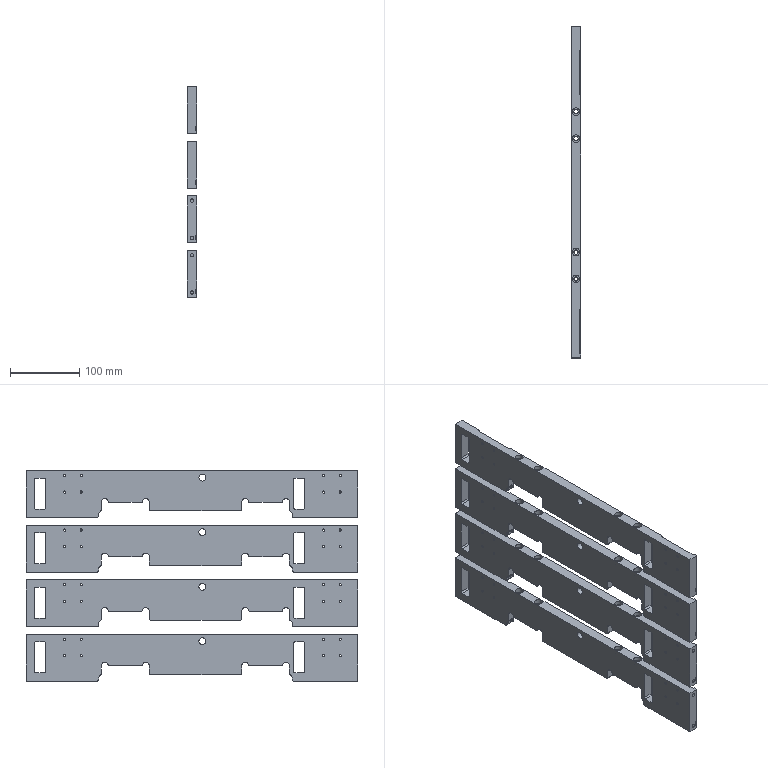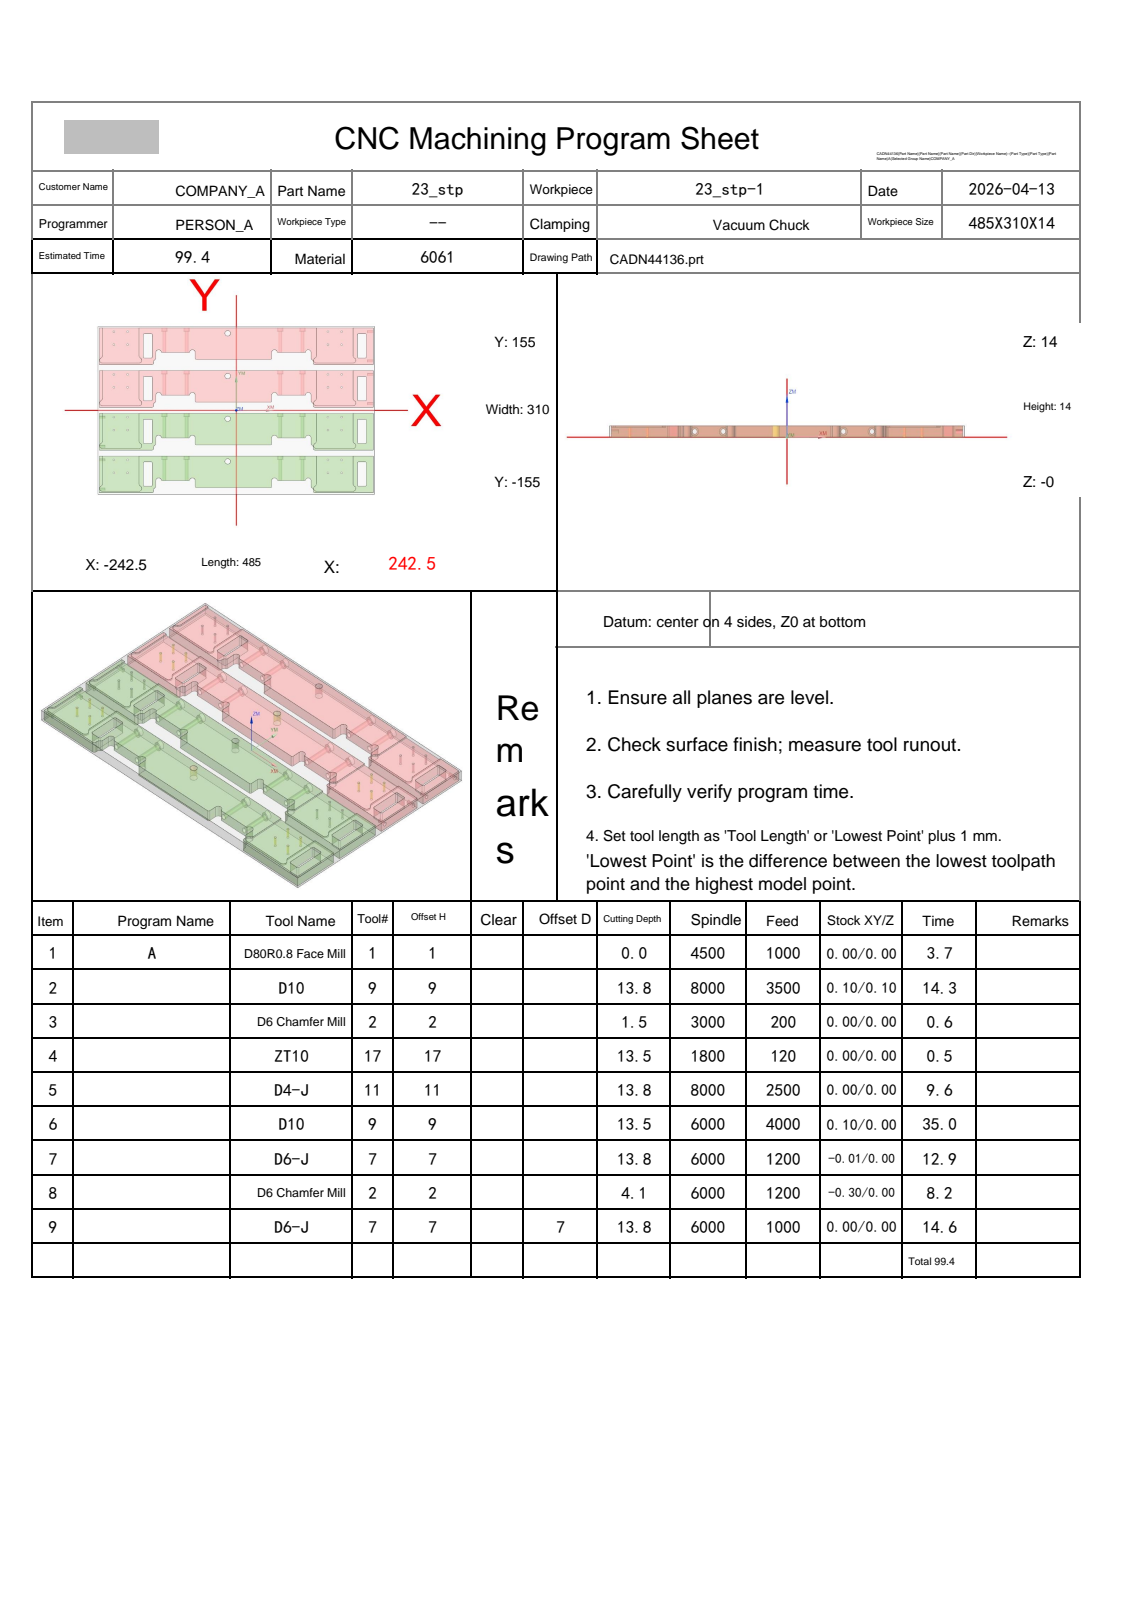NC program | NX | posted by the shop | part box 14 x 480 x 305 mm
Lines 1 to 2632 of 51894:
%
O0001
(Machine time: 100.72 MIN)
(===Total Tool:6===)
(T1=D80R0.8 Face Mill D=80.  R=0.8  D-  H01 Z=14.   )
(T9=D10     D=10.  R=0.   D-  H09 Z=0.2   )
(T2=D6 Chamfer Mill   D=6.   R=0.   D-  H02 Z=9.85  )
(T17=ZT10   D=10.  DR_a=118 D-  H17 Z=0.5   )
(T11=D4-J   D=4.   R=0.   D11 H11 Z=0.2   )
(T7=D6-J    D=6.   R=0.   D7  H07 Z=0.2   )
G80 G90 G17 G49 G40
G91 G28 Z0
M01
N1 T01 M06
(D80R0.8 Face Mill  D=80. R=0.8 H=01 ce=0.00 di=0.00)
G00 G90 G54 X-292. Y137.5 M03 S4500
G43 H01 Z34.
M08
Z16.
G01 Z14. F1000.
X-280.
X280.
Y82.5
X-280.
Y27.5
X280.
Y-27.5
X-280.
Y-82.5
X280.
Y-137.5
X-280.
X-292.
Z16.
G00 Z34.
G91 G28 Z0.0
M05
M09
G91 G28 Z0.0
M01
N2 T09 M06
(D10  D=10. R=0. H=09 ce=0.10 di=0.10)
G00 G90 G54 X-201.35 Y-115.71 M03 S8000
G43 H09 Z34.
M08
Z14.5
M03 S8000
G01 Y-110.28 Z14.31 F2800.
X-203.65 Z14.23
Y-118.65 Z13.938
X-201.35 Z13.857
Y-110.28 Z13.565
X-202.5 Z13.525
Y-109.98
M03 S8000
X-203.95 F3500.
Y-118.95
X-201.05
Y-109.98
X-202.5
Y-105.48
X-208.45
Y-123.45
X-196.55
Y-105.48
X-202.5
Y-98.48
X-215.45
Y-130.45
X-189.55
Y-98.48
X-202.5
Y-91.48
X-222.45
Y-135.84
G02 X-222.526 Y-137.45 I-17.05 J0.0
G01 X-182.474
G02 X-182.55 Y-135.84 I16.974 J1.61
G01 Y-91.48
X-202.5
Y-84.48
X-229.45
Y-135.84
G02 X-234.317 Y-144.45 I-10.05 J0.0
G01 X-170.701
X-171.032 Y-144.23
X-171.094 Y-144.189
G02 X-175.55 Y-135.84 I5.594 J8.349
G01 Y-84.48
X-202.5
Z14.525
G00 Z15.
X-201.35 Y-115.71
Z14.025
M03 S8000
G01 Y-110.28 Z13.835 F2800.
X-203.65 Z13.755
Y-118.65 Z13.463
X-201.35 Z13.382
Y-110.28 Z13.09
X-202.5 Z13.05
Y-109.98
M03 S8000
X-203.95 F3500.
Y-118.95
X-201.05
Y-109.98
X-202.5
Y-105.48
X-208.45
Y-123.45
X-196.55
Y-105.48
X-202.5
Y-98.48
X-215.45
Y-130.45
X-189.55
Y-98.48
X-202.5
Y-91.48
X-222.45
Y-135.84
G02 X-222.526 Y-137.45 I-17.05 J0.0
G01 X-182.474
G02 X-182.55 Y-135.84 I16.974 J1.61
G01 Y-91.48
X-202.5
Y-84.48
X-229.45
Y-135.84
G02 X-234.317 Y-144.45 I-10.05 J0.0
G01 X-170.701
X-171.032 Y-144.23
G02 X-175.55 Y-135.84 I5.532 J8.39
G01 Y-84.48
X-202.5
Z14.05
G00 Z14.525
X-201.35 Y-115.71
Z13.55
M03 S8000
G01 Y-110.28 Z13.36 F2800.
X-203.65 Z13.28
Y-118.65 Z12.988
X-201.35 Z12.907
Y-110.28 Z12.615
X-202.5 Z12.575
Y-109.98
M03 S8000
X-203.95 F3500.
Y-118.95
X-201.05
Y-109.98
X-202.5
Y-105.48
X-208.45
Y-123.45
X-196.55
Y-105.48
X-202.5
Y-98.48
X-215.45
Y-130.45
X-189.55
Y-98.48
X-202.5
Y-91.48
X-222.45
Y-135.84
G02 X-222.526 Y-137.45 I-17.05 J0.0
G01 X-182.474
G02 X-182.55 Y-135.84 I16.974 J1.61
G01 Y-91.48
X-202.5
Y-84.48
X-229.45
Y-135.84
G02 X-234.317 Y-144.45 I-10.05 J0.0
G01 X-170.701
X-171.032 Y-144.23
G02 X-175.55 Y-135.84 I5.532 J8.39
G01 Y-84.48
X-202.5
Z13.575
G00 Z14.05
X-201.35 Y-115.71
Z13.075
M03 S8000
G01 Y-110.28 Z12.885 F2800.
X-203.65 Z12.805
Y-118.65 Z12.513
X-201.35 Z12.432
Y-110.28 Z12.14
X-202.5 Z12.1
Y-109.98
M03 S8000
X-203.95 F3500.
Y-118.95
X-201.05
Y-109.98
X-202.5
Y-105.48
X-208.45
Y-123.45
X-196.55
Y-105.48
X-202.5
Y-98.48
X-215.45
Y-130.45
X-189.55
Y-98.48
X-202.5
Y-91.48
X-222.45
Y-135.84
G02 X-222.526 Y-137.45 I-17.05 J0.0
G01 X-182.474
G02 X-182.55 Y-135.84 I16.974 J1.61
G01 Y-91.48
X-202.5
Y-84.48
X-229.45
Y-135.84
G02 X-234.317 Y-144.45 I-10.05 J0.0
G01 X-170.701
X-171.032 Y-144.23
G02 X-175.55 Y-135.84 I5.532 J8.39
G01 Y-84.48
X-202.5
Z13.1
G00 Z34.
X-201.35 Y-36.71
Z14.5
M03 S8000
G01 Y-31.28 Z14.31 F2800.
X-203.65 Z14.23
Y-39.65 Z13.938
X-201.35 Z13.857
Y-31.28 Z13.565
X-202.5 Z13.525
Y-30.98
M03 S8000
X-203.95 F3500.
Y-39.95
X-201.05
Y-30.98
X-202.5
Y-26.48
X-208.45
Y-44.45
X-196.55
Y-26.48
X-202.5
Y-19.48
X-215.45
Y-51.45
X-189.55
Y-19.48
X-202.5
Y-12.48
X-222.45
Y-56.84
G02 X-222.526 Y-58.45 I-17.05 J0.0
G01 X-182.474
G02 X-182.55 Y-56.84 I16.974 J1.61
G01 Y-12.48
X-202.5
Y-5.48
X-229.45
Y-56.84
G02 X-234.317 Y-65.45 I-10.05 J0.0
G01 X-170.691
X-170.888 Y-65.323
G02 X-175.55 Y-56.84 I5.388 J8.483
G01 Y-5.48
X-202.5
Z14.525
G00 Z15.
X-201.35 Y-36.71
Z14.025
M03 S8000
G01 Y-31.28 Z13.835 F2800.
X-203.65 Z13.755
Y-39.65 Z13.463
X-201.35 Z13.382
Y-31.28 Z13.09
X-202.5 Z13.05
Y-30.98
M03 S8000
X-203.95 F3500.
Y-39.95
X-201.05
Y-30.98
X-202.5
Y-26.48
X-208.45
Y-44.45
X-196.55
Y-26.48
X-202.5
Y-19.48
X-215.45
Y-51.45
X-189.55
Y-19.48
X-202.5
Y-12.48
X-222.45
Y-56.84
G02 X-222.526 Y-58.45 I-17.05 J0.0
G01 X-182.474
G02 X-182.55 Y-56.84 I16.974 J1.61
G01 Y-12.48
X-202.5
Y-5.48
X-229.45
Y-56.84
G02 X-234.317 Y-65.45 I-10.05 J0.0
G01 X-170.691
X-170.888 Y-65.323
G02 X-175.55 Y-56.84 I5.388 J8.483
G01 Y-5.48
X-202.5
Z14.05
G00 Z14.525
X-201.35 Y-36.71
Z13.55
M03 S8000
G01 Y-31.28 Z13.36 F2800.
X-203.65 Z13.28
Y-39.65 Z12.988
X-201.35 Z12.907
Y-31.28 Z12.615
X-202.5 Z12.575
Y-30.98
M03 S8000
X-203.95 F3500.
Y-39.95
X-201.05
Y-30.98
X-202.5
Y-26.48
X-208.45
Y-44.45
X-196.55
Y-26.48
X-202.5
Y-19.48
X-215.45
Y-51.45
X-189.55
Y-19.48
X-202.5
Y-12.48
X-222.45
Y-56.84
G02 X-222.526 Y-58.45 I-17.05 J0.0
G01 X-182.474
G02 X-182.55 Y-56.84 I16.974 J1.61
G01 Y-12.48
X-202.5
Y-5.48
X-229.45
Y-56.84
G02 X-234.317 Y-65.45 I-10.05 J0.0
G01 X-170.691
X-170.888 Y-65.323
G02 X-175.55 Y-56.84 I5.388 J8.483
G01 Y-5.48
X-202.5
Z13.575
G00 Z14.05
X-201.35 Y-36.71
Z13.075
M03 S8000
G01 Y-31.28 Z12.885 F2800.
X-203.65 Z12.805
Y-39.65 Z12.513
X-201.35 Z12.432
Y-31.28 Z12.14
X-202.5 Z12.1
Y-30.98
M03 S8000
X-203.95 F3500.
Y-39.95
X-201.05
Y-30.98
X-202.5
Y-26.48
X-208.45
Y-44.45
X-196.55
Y-26.48
X-202.5
Y-19.48
X-215.45
Y-51.45
X-189.55
Y-19.48
X-202.5
Y-12.48
X-222.45
Y-56.84
G02 X-222.526 Y-58.45 I-17.05 J0.0
G01 X-182.474
G02 X-182.55 Y-56.84 I16.974 J1.61
G01 Y-12.48
X-202.5
Y-5.48
X-229.45
Y-56.84
G02 X-234.317 Y-65.45 I-10.05 J0.0
G01 X-170.691
X-170.888 Y-65.323
G02 X-175.55 Y-56.84 I5.388 J8.483
G01 Y-5.48
X-202.5
Z13.1
G00 Z34.
X-201.35 Y42.29
Z14.5
M03 S8000
G01 Y47.72 Z14.31 F2800.
X-203.65 Z14.23
Y39.35 Z13.938
X-201.35 Z13.857
Y47.72 Z13.565
X-202.5 Z13.525
Y48.02
M03 S8000
X-203.95 F3500.
Y39.05
X-201.05
Y48.02
X-202.5
Y52.52
X-208.45
Y34.55
X-196.55
Y52.52
X-202.5
Y59.52
X-215.45
Y27.55
X-189.55
Y59.52
X-202.5
Y66.52
X-222.45
Y22.16
G02 X-222.526 Y20.55 I-17.05 J0.0
G01 X-182.474
G02 X-182.55 Y22.16 I16.974 J1.61
G01 Y66.52
X-202.5
Y73.52
X-229.45
Y22.16
G02 X-234.317 Y13.55 I-10.05 J0.0
G01 X-170.692
X-170.818 Y13.633
X-170.856 Y13.656
G02 X-175.55 Y22.16 I5.356 J8.504
G01 Y73.52
X-202.5
Z14.525
G00 Z15.
X-201.35 Y42.29
Z14.025
M03 S8000
G01 Y47.72 Z13.835 F2800.
X-203.65 Z13.755
Y39.35 Z13.463
X-201.35 Z13.382
Y47.72 Z13.09
X-202.5 Z13.05
Y48.02
M03 S8000
X-203.95 F3500.
Y39.05
X-201.05
Y48.02
X-202.5
Y52.52
X-208.45
Y34.55
X-196.55
Y52.52
X-202.5
Y59.52
X-215.45
Y27.55
X-189.55
Y59.52
X-202.5
Y66.52
X-222.45
Y22.16
G02 X-222.526 Y20.55 I-17.05 J0.0
G01 X-182.474
G02 X-182.55 Y22.16 I16.974 J1.61
G01 Y66.52
X-202.5
Y73.52
X-229.45
Y22.16
G02 X-234.317 Y13.55 I-10.05 J0.0
G01 X-170.692
X-170.818 Y13.633
G02 X-175.55 Y22.16 I5.318 J8.528
G01 Y73.52
X-202.5
Z14.05
G00 Z14.525
X-201.35 Y42.29
Z13.55
M03 S8000
G01 Y47.72 Z13.36 F2800.
X-203.65 Z13.28
Y39.35 Z12.988
X-201.35 Z12.907
Y47.72 Z12.615
X-202.5 Z12.575
Y48.02
M03 S8000
X-203.95 F3500.
Y39.05
X-201.05
Y48.02
X-202.5
Y52.52
X-208.45
Y34.55
X-196.55
Y52.52
X-202.5
Y59.52
X-215.45
Y27.55
X-189.55
Y59.52
X-202.5
Y66.52
X-222.45
Y22.16
G02 X-222.526 Y20.55 I-17.05 J0.0
G01 X-182.474
G02 X-182.55 Y22.16 I16.974 J1.61
G01 Y66.52
X-202.5
Y73.52
X-229.45
Y22.16
G02 X-234.317 Y13.55 I-10.05 J0.0
G01 X-170.692
X-170.818 Y13.633
G02 X-175.55 Y22.16 I5.318 J8.528
G01 Y73.52
X-202.5
Z13.575
G00 Z14.05
X-201.35 Y42.29
Z13.075
M03 S8000
G01 Y47.72 Z12.885 F2800.
X-203.65 Z12.805
Y39.35 Z12.513
X-201.35 Z12.432
Y47.72 Z12.14
X-202.5 Z12.1
Y48.02
M03 S8000
X-203.95 F3500.
Y39.05
X-201.05
Y48.02
X-202.5
Y52.52
X-208.45
Y34.55
X-196.55
Y52.52
X-202.5
Y59.52
X-215.45
Y27.55
X-189.55
Y59.52
X-202.5
Y66.52
X-222.45
Y22.16
G02 X-222.526 Y20.55 I-17.05 J0.0
G01 X-182.474
G02 X-182.55 Y22.16 I16.974 J1.61
G01 Y66.52
X-202.5
Y73.52
X-229.45
Y22.16
G02 X-233.984 Y13.76 I-10.05 J0.0
X-234.317 Y13.55 I-5.516 J8.401
G01 X-170.692
X-170.818 Y13.633
G02 X-175.55 Y22.16 I5.318 J8.528
G01 Y73.52
X-202.5
Z13.1
G00 Z34.
X-201.35 Y121.29
Z14.5
M03 S8000
G01 Y126.72 Z14.31 F2800.
X-203.65 Z14.23
Y118.35 Z13.938
X-201.35 Z13.857
Y126.72 Z13.565
X-202.5 Z13.525
Y127.02
M03 S8000
X-203.95 F3500.
Y118.05
X-201.05
Y127.02
X-202.5
Y131.52
X-208.45
Y113.55
X-196.55
Y131.52
X-202.5
Y138.52
X-215.45
Y106.55
X-189.55
Y138.52
X-202.5
Y145.52
X-222.45
Y101.16
G02 X-222.526 Y99.55 I-17.05 J0.0
G01 X-182.474
G02 X-182.55 Y101.16 I16.974 J1.61
G01 Y145.52
X-202.5
Y152.52
X-229.055
X-229.45
Y101.16
G02 X-234.317 Y92.55 I-10.05 J0.0
G01 X-170.701
X-171.061 Y92.789
G02 X-175.55 Y101.16 I5.561 J8.371
G01 Y152.52
X-202.5
Z14.525
G00 Z15.
X-201.35 Y121.29
Z14.025
M03 S8000
G01 Y126.72 Z13.835 F2800.
X-203.65 Z13.755
Y118.35 Z13.463
X-201.35 Z13.382
Y126.72 Z13.09
X-202.5 Z13.05
Y127.02
M03 S8000
X-203.95 F3500.
Y118.05
X-201.05
Y127.02
X-202.5
Y131.52
X-208.45
Y113.55
X-196.55
Y131.52
X-202.5
Y138.52
X-215.45
Y106.55
X-189.55
Y138.52
X-202.5
Y145.52
X-222.45
Y101.16
G02 X-222.526 Y99.55 I-17.05 J0.0
G01 X-182.474
G02 X-182.55 Y101.16 I16.974 J1.61
G01 Y145.52
X-202.5
Y152.52
X-229.055
X-229.45
Y101.16
G02 X-234.317 Y92.55 I-10.05 J0.0
G01 X-170.701
X-171.06 Y92.788
G02 X-175.55 Y101.16 I5.56 J8.372
G01 Y152.52
X-202.5
Z14.05
G00 Z14.525
X-201.35 Y121.29
Z13.55
M03 S8000
G01 Y126.72 Z13.36 F2800.
X-203.65 Z13.28
Y118.35 Z12.988
X-201.35 Z12.907
Y126.72 Z12.615
X-202.5 Z12.575
Y127.02
M03 S8000
X-203.95 F3500.
Y118.05
X-201.05
Y127.02
X-202.5
Y131.52
X-208.45
Y113.55
X-196.55
Y131.52
X-202.5
Y138.52
X-215.45
Y106.55
X-189.55
Y138.52
X-202.5
Y145.52
X-222.45
Y101.16
G02 X-222.526 Y99.55 I-17.05 J0.0
G01 X-182.474
G02 X-182.55 Y101.16 I16.974 J1.61
G01 Y145.52
X-202.5
Y152.52
X-229.055
X-229.45
Y101.16
G02 X-234.317 Y92.55 I-10.05 J0.0
G01 X-170.701
X-171.06 Y92.788
G02 X-175.55 Y101.16 I5.56 J8.372
G01 Y152.52
X-202.5
Z13.575
G00 Z14.05
X-201.35 Y121.29
Z13.075
M03 S8000
G01 Y126.72 Z12.885 F2800.
X-203.65 Z12.805
Y118.35 Z12.513
X-201.35 Z12.432
Y126.72 Z12.14
X-202.5 Z12.1
Y127.02
M03 S8000
X-203.95 F3500.
Y118.05
X-201.05
Y127.02
X-202.5
Y131.52
X-208.45
Y113.55
X-196.55
Y131.52
X-202.5
Y138.52
X-215.45
Y106.55
X-189.55
Y138.52
X-202.5
Y145.52
X-222.45
Y101.16
G02 X-222.526 Y99.55 I-17.05 J0.0
G01 X-182.474
G02 X-182.55 Y101.16 I16.974 J1.61
G01 Y145.52
X-202.5
Y152.52
X-229.055
X-229.45
Y101.16
G02 X-234.317 Y92.55 I-10.05 J0.0
G01 X-170.701
X-171.06 Y92.788
G02 X-175.55 Y101.16 I5.56 J8.372
G01 Y152.52
X-202.5
Z13.1
G00 Z34.
X173.65 Y121.29
Z14.5
M03 S8000
G01 Y126.72 Z14.31 F2800.
X171.35 Z14.23
Y118.35 Z13.938
X173.65 Z13.857
Y126.72 Z13.565
X172.5 Z13.525
Y127.02
M03 S8000
X171.05 F3500.
Y118.05
X173.95
Y127.02
X172.5
Y131.52
X166.55
Y113.55
X178.45
Y131.52
X172.5
Y138.52
X159.55
Y106.55
X185.45
Y138.52
X172.5
Y145.52
X152.55
Y101.16
G02 X152.474 Y99.55 I-17.05 J0.0
G01 X192.526
G02 X192.45 Y101.16 I16.974 J1.61
G01 Y145.52
X172.5
Y152.52
X145.55
Y101.16
G02 X140.683 Y92.55 I-10.05 J0.0
G01 X204.313
X204.164 Y92.644
G02 X199.45 Y101.16 I5.336 J8.516
G01 Y152.52
X172.5
Z14.525
G00 Z15.
X173.65 Y121.29
Z14.025
M03 S8000
G01 Y126.72 Z13.835 F2800.
X171.35 Z13.755
Y118.35 Z13.463
X173.65 Z13.382
Y126.72 Z13.09
X172.5 Z13.05
Y127.02
M03 S8000
X171.05 F3500.
Y118.05
X173.95
Y127.02
X172.5
Y131.52
X166.55
Y113.55
X178.45
Y131.52
X172.5
Y138.52
X159.55
Y106.55
X185.45
Y138.52
X172.5
Y145.52
X152.55
Y101.16
G02 X152.474 Y99.55 I-17.05 J0.0
G01 X192.526
G02 X192.45 Y101.16 I16.974 J1.61
G01 Y145.52
X172.5
Y152.52
X145.55
Y101.16
G02 X140.683 Y92.55 I-10.05 J0.0
G01 X204.313
X204.164 Y92.644
G02 X199.45 Y101.16 I5.336 J8.516
G01 Y152.52
X172.5
Z14.05
G00 Z14.525
X173.65 Y121.29
Z13.55
M03 S8000
G01 Y126.72 Z13.36 F2800.
X171.35 Z13.28
Y118.35 Z12.988
X173.65 Z12.907
Y126.72 Z12.615
X172.5 Z12.575
Y127.02
M03 S8000
X171.05 F3500.
Y118.05
X173.95
Y127.02
X172.5
Y131.52
X166.55
Y113.55
X178.45
Y131.52
X172.5
Y138.52
X159.55
Y106.55
X185.45
Y138.52
X172.5
Y145.52
X152.55
Y101.16
G02 X152.474 Y99.55 I-17.05 J0.0
G01 X192.526
G02 X192.45 Y101.16 I16.974 J1.61
G01 Y145.52
X172.5
Y152.52
X145.55
Y101.16
G02 X140.683 Y92.55 I-10.05 J0.0
G01 X204.313
X204.164 Y92.644
G02 X199.45 Y101.16 I5.336 J8.516
G01 Y152.52
X172.5
Z13.575
G00 Z14.05
X173.65 Y121.29
Z13.075
M03 S8000
G01 Y126.72 Z12.885 F2800.
X171.35 Z12.805
Y118.35 Z12.513
X173.65 Z12.432
Y126.72 Z12.14
X172.5 Z12.1
Y127.02
M03 S8000
X171.05 F3500.
Y118.05
X173.95
Y127.02
X172.5
Y131.52
X166.55
Y113.55
X178.45
Y131.52
X172.5
Y138.52
X159.55
Y106.55
X185.45
Y138.52
X172.5
Y145.52
X152.55
Y101.16
G02 X152.474 Y99.55 I-17.05 J0.0
G01 X192.526
G02 X192.45 Y101.16 I16.974 J1.61
G01 Y145.52
X172.5
Y152.52
X145.55
Y101.16
G02 X140.683 Y92.55 I-10.05 J0.0
G01 X204.313
X204.164 Y92.644
G02 X199.45 Y101.16 I5.336 J8.516
G01 Y152.52
X172.5
Z13.1
G00 Z34.
X173.65 Y42.29
Z14.5
M03 S8000
G01 Y47.72 Z14.31 F2800.
X171.35 Z14.23
Y39.35 Z13.938
X173.65 Z13.857
Y47.72 Z13.565
X172.5 Z13.525
Y48.02
M03 S8000
X171.05 F3500.
Y39.05
X173.95
Y48.02
X172.5
Y52.52
X166.55
Y34.55
X178.45
Y52.52
X172.5
Y59.52
X159.55
Y27.55
X185.45
Y59.52
X172.5
Y66.52
X152.55
Y22.16
G02 X152.474 Y20.55 I-17.05 J0.0
G01 X192.526
G02 X192.45 Y22.16 I16.974 J1.61
G01 Y66.52
X172.5
Y73.52
X145.55
Y22.16
G02 X140.683 Y13.55 I-10.05 J0.0
G01 X204.317
G02 X199.45 Y22.16 I5.183 J8.61
G01 Y73.52
X172.5
Z14.525
G00 Z15.
X173.65 Y42.29
Z14.025
M03 S8000
G01 Y47.72 Z13.835 F2800.
X171.35 Z13.755
Y39.35 Z13.463
X173.65 Z13.382
Y47.72 Z13.09
X172.5 Z13.05
Y48.02
M03 S8000
X171.05 F3500.
Y39.05
X173.95
Y48.02
X172.5
Y52.52
X166.55
Y34.55
X178.45
Y52.52
X172.5
Y59.52
X159.55
Y27.55
X185.45
Y59.52
X172.5
Y66.52
X152.55
Y22.16
G02 X152.474 Y20.55 I-17.05 J0.0
G01 X192.526
G02 X192.45 Y22.16 I16.974 J1.61
G01 Y66.52
X172.5
Y73.52
X145.55
Y22.16
G02 X140.683 Y13.55 I-10.05 J0.0
G01 X204.317
G02 X199.45 Y22.16 I5.183 J8.61
G01 Y73.52
X172.5
Z14.05
G00 Z14.525
X173.65 Y42.29
Z13.55
M03 S8000
G01 Y47.72 Z13.36 F2800.
X171.35 Z13.28
Y39.35 Z12.988
X173.65 Z12.907
Y47.72 Z12.615
X172.5 Z12.575
Y48.02
M03 S8000
X171.05 F3500.
Y39.05
X173.95
Y48.02
X172.5
Y52.52
X166.55
Y34.55
X178.45
Y52.52
X172.5
Y59.52
X159.55
Y27.55
X185.45
Y59.52
X172.5
Y66.52
X152.55
Y22.16
G02 X152.474 Y20.55 I-17.05 J0.0
G01 X192.526
G02 X192.45 Y22.16 I16.974 J1.61
G01 Y66.52
X172.5
Y73.52
X145.55
Y22.16
G02 X140.683 Y13.55 I-10.05 J0.0
G01 X204.317
G02 X199.45 Y22.16 I5.183 J8.61
G01 Y73.52
X172.5
Z13.575
G00 Z14.05
X173.65 Y42.29
Z13.075
M03 S8000
G01 Y47.72 Z12.885 F2800.
X171.35 Z12.805
Y39.35 Z12.513
X173.65 Z12.432
Y47.72 Z12.14
X172.5 Z12.1
Y48.02
M03 S8000
X171.05 F3500.
Y39.05
X173.95
Y48.02
X172.5
Y52.52
X166.55
Y34.55
X178.45
Y52.52
X172.5
Y59.52
X159.55
Y27.55
X185.45
Y59.52
X172.5
Y66.52
X152.55
Y22.16
G02 X152.474 Y20.55 I-17.05 J0.0
G01 X192.526
G02 X192.45 Y22.16 I16.974 J1.61
G01 Y66.52
X172.5
Y73.52
X145.55
Y22.16
G02 X141.838 Y14.361 I-10.05 J0.0
X140.683 Y13.55 I-6.338 J7.8
G01 X204.317
G02 X199.45 Y22.16 I5.183 J8.61
G01 Y73.52
X172.5
Z13.1
G00 Z34.
X173.65 Y-36.71
Z14.5
M03 S8000
G01 Y-31.28 Z14.31 F2800.
X171.35 Z14.23
Y-39.65 Z13.938
X173.65 Z13.857
Y-31.28 Z13.565
X172.5 Z13.525
Y-30.98
M03 S8000
X171.05 F3500.
Y-39.95
X173.95
Y-30.98
X172.5
Y-26.48
X166.55
Y-44.45
X178.45
Y-26.48
X172.5
Y-19.48
X159.55
Y-51.45
X185.45
Y-19.48
X172.5
Y-12.48
X152.55
Y-56.84
G02 X152.474 Y-58.45 I-17.05 J0.0
G01 X192.526
G02 X192.45 Y-56.84 I16.974 J1.61
G01 Y-12.48
X172.5
Y-5.48
X145.55
Y-56.84
G02 X140.683 Y-65.45 I-10.05 J0.0
G01 X204.317
G02 X199.45 Y-56.84 I5.183 J8.61
G01 Y-5.48
X172.5
Z14.525
G00 Z15.
X173.65 Y-36.71
Z14.025
M03 S8000
G01 Y-31.28 Z13.835 F2800.
X171.35 Z13.755
Y-39.65 Z13.463
X173.65 Z13.382
Y-31.28 Z13.09
X172.5 Z13.05
Y-30.98
M03 S8000
X171.05 F3500.
Y-39.95
X173.95
Y-30.98
X172.5
Y-26.48
X166.55
Y-44.45
X178.45
Y-26.48
X172.5
Y-19.48
X159.55
Y-51.45
X185.45
Y-19.48
X172.5
Y-12.48
X152.55
Y-56.84
G02 X152.474 Y-58.45 I-17.05 J0.0
G01 X192.526
G02 X192.45 Y-56.84 I16.974 J1.61
G01 Y-12.48
X172.5
Y-5.48
X145.55
Y-56.84
G02 X140.683 Y-65.45 I-10.05 J0.0
G01 X204.317
G02 X199.45 Y-56.84 I5.183 J8.61
G01 Y-5.48
X172.5
Z14.05
G00 Z14.525
X173.65 Y-36.71
Z13.55
M03 S8000
G01 Y-31.28 Z13.36 F2800.
X171.35 Z13.28
Y-39.65 Z12.988
X173.65 Z12.907
Y-31.28 Z12.615
X172.5 Z12.575
Y-30.98
M03 S8000
X171.05 F3500.
Y-39.95
X173.95
Y-30.98
X172.5
Y-26.48
X166.55
Y-44.45
X178.45
Y-26.48
X172.5
Y-19.48
X159.55
Y-51.45
X185.45
Y-19.48
X172.5
Y-12.48
X152.55
Y-56.84
G02 X152.474 Y-58.45 I-17.05 J0.0
G01 X192.526
G02 X192.45 Y-56.84 I16.974 J1.61
G01 Y-12.48
X172.5
Y-5.48
X145.55
Y-56.84
G02 X140.683 Y-65.45 I-10.05 J0.0
G01 X204.317
G02 X199.45 Y-56.84 I5.183 J8.61
G01 Y-5.48
X172.5
Z13.575
G00 Z14.05
X173.65 Y-36.71
Z13.075
M03 S8000
G01 Y-31.28 Z12.885 F2800.
X171.35 Z12.805
Y-39.65 Z12.513
X173.65 Z12.432
Y-31.28 Z12.14
X172.5 Z12.1
Y-30.98
M03 S8000
X171.05 F3500.
Y-39.95
X173.95
Y-30.98
X172.5
Y-26.48
X166.55
Y-44.45
X178.45
Y-26.48
X172.5
Y-19.48
X159.55
Y-51.45
X185.45
Y-19.48
X172.5
Y-12.48
X152.55
Y-56.84
G02 X152.474 Y-58.45 I-17.05 J0.0
G01 X192.526
G02 X192.45 Y-56.84 I16.974 J1.61
G01 Y-12.48
X172.5
Y-5.48
X145.55
Y-56.84
G02 X140.683 Y-65.45 I-10.05 J0.0
G01 X204.317
G02 X199.45 Y-56.84 I5.183 J8.61
G01 Y-5.48
X172.5
Z13.1
G00 Z34.
X173.65 Y-115.71
Z14.5
M03 S8000
G01 Y-110.28 Z14.31 F2800.
X171.35 Z14.23
Y-118.65 Z13.938
X173.65 Z13.857
Y-110.28 Z13.565
X172.5 Z13.525
Y-109.98
M03 S8000
X171.05 F3500.
Y-118.95
X173.95
Y-109.98
X172.5
Y-105.48
X166.55
Y-123.45
X178.45
Y-105.48
X172.5
Y-98.48
X159.55
Y-130.45
X185.45
Y-98.48
X172.5
Y-91.48
X152.55
Y-135.84
G02 X152.474 Y-137.45 I-17.05 J0.0
G01 X192.526
G02 X192.45 Y-135.84 I16.974 J1.61
G01 Y-91.48
X172.5
Y-84.48
X145.55
Y-135.84
G02 X140.683 Y-144.45 I-10.05 J0.0
G01 X204.317
G02 X199.45 Y-135.84 I5.183 J8.61
G01 Y-84.48
X172.5
Z14.525
G00 Z15.
X173.65 Y-115.71
Z14.025
M03 S8000
G01 Y-110.28 Z13.835 F2800.
X171.35 Z13.755
Y-118.65 Z13.463
X173.65 Z13.382
Y-110.28 Z13.09
X172.5 Z13.05
Y-109.98
M03 S8000
X171.05 F3500.
Y-118.95
X173.95
Y-109.98
X172.5
Y-105.48
X166.55
Y-123.45
X178.45
Y-105.48
X172.5
Y-98.48
X159.55
Y-130.45
X185.45
Y-98.48
X172.5
Y-91.48
X152.55
Y-135.84
G02 X152.474 Y-137.45 I-17.05 J0.0
G01 X192.526
G02 X192.45 Y-135.84 I16.974 J1.61
G01 Y-91.48
X172.5
Y-84.48
X145.55
Y-135.84
G02 X140.683 Y-144.45 I-10.05 J0.0
G01 X204.317
G02 X199.45 Y-135.84 I5.183 J8.61
G01 Y-84.48
X172.5
Z14.05
G00 Z14.525
X173.65 Y-115.71
Z13.55
M03 S8000
G01 Y-110.28 Z13.36 F2800.
X171.35 Z13.28
Y-118.65 Z12.988
X173.65 Z12.907
Y-110.28 Z12.615
X172.5 Z12.575
Y-109.98
M03 S8000
X171.05 F3500.
Y-118.95
X173.95
Y-109.98
X172.5
Y-105.48
X166.55
Y-123.45
X178.45
Y-105.48
X172.5
Y-98.48
X159.55
Y-130.45
X185.45
Y-98.48
X172.5
Y-91.48
X152.55
Y-135.84
G02 X152.474 Y-137.45 I-17.05 J0.0
G01 X192.526
G02 X192.45 Y-135.84 I16.974 J1.61
G01 Y-91.48
X172.5
Y-84.48
X145.55
Y-135.84
G02 X140.683 Y-144.45 I-10.05 J0.0
G01 X204.317
G02 X199.45 Y-135.84 I5.183 J8.61
G01 Y-84.48
X172.5
Z13.575
G00 Z14.05
X173.65 Y-115.71
Z13.075
M03 S8000
G01 Y-110.28 Z12.885 F2800.
X171.35 Z12.805
Y-118.65 Z12.513
X173.65 Z12.432
Y-110.28 Z12.14
X172.5 Z12.1
Y-109.98
M03 S8000
X171.05 F3500.
Y-118.95
X173.95
Y-109.98
X172.5
Y-105.48
X166.55
Y-123.45
X178.45
Y-105.48
X172.5
Y-98.48
X159.55
Y-130.45
X185.45
Y-98.48
X172.5
Y-91.48
X152.55
Y-135.84
G02 X152.474 Y-137.45 I-17.05 J0.0
G01 X192.526
G02 X192.45 Y-135.84 I16.974 J1.61
G01 Y-91.48
X172.5
Y-84.48
X145.55
Y-135.84
G02 X140.683 Y-144.45 I-10.05 J0.0
G01 X204.317
G02 X199.45 Y-135.84 I5.183 J8.61
G01 Y-84.48
X172.5
Z13.1
G00 Z34.
G00 G90 X-152.1 Y-117.75 M03 S8000
Z34.
Z14.5
G01 Y-100.35 Z14.394 F2500.
X-157.9 Z14.359
Y-135.15 Z14.148
X-152.1 Z14.113
Y-100.35 Z13.901
X-157.9 Z13.866
Y-135.15 Z13.655
X-152.1 Z13.619
Y-100.35 Z13.408
X-157.9 Z13.373
Y-135.15 Z13.162
X-152.1 Z13.126
Y-100.35 Z12.915
X-157.9 Z12.88
Y-135.15 Z12.668
X-152.1 Z12.633
Y-100.35 Z12.422
X-157.9 Z12.387
Y-135.15 Z12.175
X-152.1 Z12.14
Y-100.35 Z11.929
X-157.9 Z11.894
Y-135.15 Z11.682
X-152.1 Z11.647
Y-100.35 Z11.436
X-157.9 Z11.4
Y-135.15 Z11.189
X-152.1 Z11.154
Y-100.35 Z10.943
X-157.9 Z10.907
Y-135.15 Z10.696
X-152.1 Z10.661
Y-100.35 Z10.45
X-157.9 Z10.414
Y-135.15 Z10.203
X-152.1 Z10.168
Y-100.35 Z9.956
X-157.9 Z9.921
Y-135.15 Z9.71
X-152.1 Z9.675
Y-100.35 Z9.463
X-157.9 Z9.428
Y-135.15 Z9.217
X-152.1 Z9.182
Y-100.35 Z8.97
X-157.9 Z8.935
Y-135.15 Z8.724
X-152.1 Z8.688
Y-100.35 Z8.477
X-157.9 Z8.442
Y-135.15 Z8.231
X-152.1 Z8.195
Y-100.35 Z7.984
X-157.9 Z7.949
Y-135.15 Z7.737
X-152.1 Z7.702
Y-100.35 Z7.491
X-157.9 Z7.456
Y-135.15 Z7.244
X-152.1 Z7.209
Y-100.35 Z6.998
X-157.9 Z6.963
Y-135.15 Z6.751
X-152.1 Z6.716
Y-100.35 Z6.505
X-157.9 Z6.469
Y-135.15 Z6.258
X-152.1 Z6.223
Y-100.35 Z6.012
X-157.9 Z5.976
Y-135.15 Z5.765
X-152.1 Z5.73
Y-100.35 Z5.518
X-157.9 Z5.483
Y-135.15 Z5.272
X-152.1 Z5.237
Y-100.35 Z5.025
X-157.9 Z4.99
Y-135.15 Z4.779
X-152.1 Z4.744
Y-100.35 Z4.532
X-157.9 Z4.497
Y-135.15 Z4.286
X-152.1 Z4.25
Y-100.35 Z4.039
X-157.9 Z4.004
Y-135.15 Z3.793
X-152.1 Z3.757
Y-100.35 Z3.546
X-157.9 Z3.511
Y-135.15 Z3.3
X-152.1 Z3.264
Y-100.35 Z3.053
X-157.9 Z3.018
Y-135.15 Z2.806
X-152.1 Z2.771
Y-100.35 Z2.56
X-157.9 Z2.525
Y-135.15 Z2.313
X-152.1 Z2.278
Y-100.35 Z2.067
X-157.9 Z2.032
Y-135.15 Z1.82
X-152.1 Z1.785
Y-100.35 Z1.574
X-157.9 Z1.538
Y-135.15 Z1.327
X-152.1 Z1.292
Y-100.35 Z1.081
X-157.9 Z1.045
Y-135.15 Z.834
X-152.1 Z.799
Y-100.35 Z.587
X-157.9 Z.552
Y-135.15 Z.341
X-152.1 Z.306
Y-117.75 Z.2
Y-100.35
X-157.9
Y-135.15
X-152.1
Y-117.75
Y-117.25
Z1.2
G00 Z34.
X-157.9 Y-38.75
Z14.5
G01 Y-56.15 Z14.394
X-152.1 Z14.359
Y-21.35 Z14.148
X-157.9 Z14.113
Y-56.15 Z13.901
X-152.1 Z13.866
Y-21.35 Z13.655
X-157.9 Z13.619
Y-56.15 Z13.408
X-152.1 Z13.373
Y-21.35 Z13.162
X-157.9 Z13.126
Y-56.15 Z12.915
X-152.1 Z12.88
Y-21.35 Z12.668
X-157.9 Z12.633
Y-56.15 Z12.422
X-152.1 Z12.387
Y-21.35 Z12.175
X-157.9 Z12.14
Y-56.15 Z11.929
X-152.1 Z11.894
Y-21.35 Z11.682
X-157.9 Z11.647
Y-56.15 Z11.436
X-152.1 Z11.4
Y-21.35 Z11.189
X-157.9 Z11.154
Y-56.15 Z10.943
X-152.1 Z10.907
Y-21.35 Z10.696
X-157.9 Z10.661
Y-56.15 Z10.45
X-152.1 Z10.414
Y-21.35 Z10.203
X-157.9 Z10.168
Y-56.15 Z9.956
X-152.1 Z9.921
Y-21.35 Z9.71
X-157.9 Z9.675
Y-56.15 Z9.463
X-152.1 Z9.428
Y-21.35 Z9.217
X-157.9 Z9.182
Y-56.15 Z8.97
X-152.1 Z8.935
Y-21.35 Z8.724
X-157.9 Z8.688
Y-56.15 Z8.477
X-152.1 Z8.442
Y-21.35 Z8.231
X-157.9 Z8.195
Y-56.15 Z7.984
X-152.1 Z7.949
Y-21.35 Z7.737
X-157.9 Z7.702
Y-56.15 Z7.491
X-152.1 Z7.456
Y-21.35 Z7.244
X-157.9 Z7.209
Y-56.15 Z6.998
X-152.1 Z6.963
Y-21.35 Z6.751
X-157.9 Z6.716
Y-56.15 Z6.505
X-152.1 Z6.469
Y-21.35 Z6.258
X-157.9 Z6.223
Y-56.15 Z6.012
X-152.1 Z5.976
Y-21.35 Z5.765
X-157.9 Z5.73
Y-56.15 Z5.518
X-152.1 Z5.483
Y-21.35 Z5.272
X-157.9 Z5.237
Y-56.15 Z5.025
X-152.1 Z4.99
Y-21.35 Z4.779
X-157.9 Z4.744
Y-56.15 Z4.532
X-152.1 Z4.497
Y-21.35 Z4.286
X-157.9 Z4.25
Y-56.15 Z4.039
X-152.1 Z4.004
Y-21.35 Z3.793
X-157.9 Z3.757
Y-56.15 Z3.546
X-152.1 Z3.511
Y-21.35 Z3.3
X-157.9 Z3.264
Y-56.15 Z3.053
X-152.1 Z3.018
Y-21.35 Z2.806
X-157.9 Z2.771
Y-56.15 Z2.56
X-152.1 Z2.525
Y-21.35 Z2.313
X-157.9 Z2.278
Y-56.15 Z2.067
X-152.1 Z2.032
Y-21.35 Z1.82
X-157.9 Z1.785
Y-56.15 Z1.574
X-152.1 Z1.538
Y-21.35 Z1.327
X-157.9 Z1.292
Y-56.15 Z1.081
X-152.1 Z1.045
Y-21.35 Z.834
X-157.9 Z.799
Y-56.15 Z.587
X-152.1 Z.552
Y-21.35 Z.341
X-157.9 Z.306
Y-38.75 Z.2
Y-56.15
X-152.1
Y-21.35
X-157.9
Y-38.75
Y-39.25
Z1.2
G00 Z34.
Y40.25
Z14.5
G01 Y22.85 Z14.394
X-152.1 Z14.359
Y57.65 Z14.148
X-157.9 Z14.113
Y22.85 Z13.901
X-152.1 Z13.866
Y57.65 Z13.655
X-157.9 Z13.619
Y22.85 Z13.408
X-152.1 Z13.373
Y57.65 Z13.162
X-157.9 Z13.126
Y22.85 Z12.915
X-152.1 Z12.88
Y57.65 Z12.668
X-157.9 Z12.633
Y22.85 Z12.422
X-152.1 Z12.387
Y57.65 Z12.175
X-157.9 Z12.14
Y22.85 Z11.929
X-152.1 Z11.894
Y57.65 Z11.682
X-157.9 Z11.647
Y22.85 Z11.436
X-152.1 Z11.4
Y57.65 Z11.189
X-157.9 Z11.154
Y22.85 Z10.943
X-152.1 Z10.907
Y57.65 Z10.696
X-157.9 Z10.661
Y22.85 Z10.45
X-152.1 Z10.414
Y57.65 Z10.203
X-157.9 Z10.168
Y22.85 Z9.956
X-152.1 Z9.921
Y57.65 Z9.71
X-157.9 Z9.675
Y22.85 Z9.463
X-152.1 Z9.428
Y57.65 Z9.217
X-157.9 Z9.182
Y22.85 Z8.97
X-152.1 Z8.935
Y57.65 Z8.724
X-157.9 Z8.688
Y22.85 Z8.477
X-152.1 Z8.442
Y57.65 Z8.231
X-157.9 Z8.195
Y22.85 Z7.984
X-152.1 Z7.949
Y57.65 Z7.737
X-157.9 Z7.702
Y22.85 Z7.491
X-152.1 Z7.456
Y57.65 Z7.244
X-157.9 Z7.209
Y22.85 Z6.998
X-152.1 Z6.963
Y57.65 Z6.751
X-157.9 Z6.716
Y22.85 Z6.505
X-152.1 Z6.469
Y57.65 Z6.258
X-157.9 Z6.223
Y22.85 Z6.012
X-152.1 Z5.976
Y57.65 Z5.765
X-157.9 Z5.73
Y22.85 Z5.518
X-152.1 Z5.483
Y57.65 Z5.272
X-157.9 Z5.237
Y22.85 Z5.025
X-152.1 Z4.99
Y57.65 Z4.779
X-157.9 Z4.744
Y22.85 Z4.532
X-152.1 Z4.497
Y57.65 Z4.286
X-157.9 Z4.25
Y22.85 Z4.039
X-152.1 Z4.004
Y57.65 Z3.793
X-157.9 Z3.757
Y22.85 Z3.546
X-152.1 Z3.511
Y57.65 Z3.3
X-157.9 Z3.264
Y22.85 Z3.053
X-152.1 Z3.018
Y57.65 Z2.806
X-157.9 Z2.771
Y22.85 Z2.56
X-152.1 Z2.525
Y57.65 Z2.313
X-157.9 Z2.278
Y22.85 Z2.067
X-152.1 Z2.032
Y57.65 Z1.82
X-157.9 Z1.785
Y22.85 Z1.574
X-152.1 Z1.538
Y57.65 Z1.327
X-157.9 Z1.292
Y22.85 Z1.081
X-152.1 Z1.045
Y57.65 Z.834
X-157.9 Z.799
Y22.85 Z.587
X-152.1 Z.552
Y57.65 Z.341
X-157.9 Z.306
Y40.25 Z.2
Y22.85
X-152.1
Y57.65
X-157.9
Y40.25
Y39.75
Z1.2
G00 Z34.
Y119.25
Z14.5
G01 Y101.85 Z14.394
X-152.1 Z14.359
Y136.65 Z14.148
X-157.9 Z14.113
Y101.85 Z13.901
X-152.1 Z13.866
Y136.65 Z13.655
X-157.9 Z13.619
Y101.85 Z13.408
X-152.1 Z13.373
Y136.65 Z13.162
X-157.9 Z13.126
Y101.85 Z12.915
X-152.1 Z12.88
Y136.65 Z12.668
X-157.9 Z12.633
Y101.85 Z12.422
X-152.1 Z12.387
Y136.65 Z12.175
X-157.9 Z12.14
Y101.85 Z11.929
X-152.1 Z11.894
Y136.65 Z11.682
X-157.9 Z11.647
Y101.85 Z11.436
X-152.1 Z11.4
Y136.65 Z11.189
X-157.9 Z11.154
Y101.85 Z10.943
X-152.1 Z10.907
Y136.65 Z10.696
X-157.9 Z10.661
Y101.85 Z10.45
X-152.1 Z10.414
Y136.65 Z10.203
X-157.9 Z10.168
Y101.85 Z9.956
X-152.1 Z9.921
Y136.65 Z9.71
X-157.9 Z9.675
Y101.85 Z9.463
X-152.1 Z9.428
Y136.65 Z9.217
X-157.9 Z9.182
Y101.85 Z8.97
X-152.1 Z8.935
Y136.65 Z8.724
X-157.9 Z8.688
Y101.85 Z8.477
X-152.1 Z8.442
Y136.65 Z8.231
X-157.9 Z8.195
Y101.85 Z7.984
X-152.1 Z7.949
Y136.65 Z7.737
X-157.9 Z7.702
Y101.85 Z7.491
X-152.1 Z7.456
Y136.65 Z7.244
X-157.9 Z7.209
Y101.85 Z6.998
X-152.1 Z6.963
Y136.65 Z6.751
X-157.9 Z6.716
Y101.85 Z6.505
X-152.1 Z6.469
Y136.65 Z6.258
X-157.9 Z6.223
Y101.85 Z6.012
X-152.1 Z5.976
Y136.65 Z5.765
X-157.9 Z5.73
Y101.85 Z5.518
X-152.1 Z5.483
Y136.65 Z5.272
X-157.9 Z5.237
Y101.85 Z5.025
X-152.1 Z4.99
Y136.65 Z4.779
X-157.9 Z4.744
Y101.85 Z4.532
X-152.1 Z4.497
Y136.65 Z4.286
X-157.9 Z4.25
Y101.85 Z4.039
X-152.1 Z4.004
Y136.65 Z3.793
X-157.9 Z3.757
Y101.85 Z3.546
X-152.1 Z3.511
Y136.65 Z3.3
X-157.9 Z3.264
Y101.85 Z3.053
X-152.1 Z3.018
Y136.65 Z2.806
X-157.9 Z2.771
Y101.85 Z2.56
X-152.1 Z2.525
Y136.65 Z2.313
X-157.9 Z2.278
Y101.85 Z2.067
X-152.1 Z2.032
Y136.65 Z1.82
X-157.9 Z1.785
Y101.85 Z1.574
X-152.1 Z1.538
Y136.65 Z1.327
X-157.9 Z1.292
Y101.85 Z1.081
X-152.1 Z1.045
Y136.65 Z.834
X-157.9 Z.799
Y101.85 Z.587
X-152.1 Z.552
Y136.65 Z.341
X-157.9 Z.306
Y119.25 Z.2
Y101.85
X-152.1
Y136.65
X-157.9
Y119.25
Y118.75
Z1.2
G00 Z34.
X222.9 Y119.25
Z14.5
G01 Y136.65 Z14.394
X217.1 Z14.359
Y101.85 Z14.148
X222.9 Z14.113
Y136.65 Z13.901
X217.1 Z13.866
Y101.85 Z13.655
X222.9 Z13.619
Y136.65 Z13.408
X217.1 Z13.373
Y101.85 Z13.162
X222.9 Z13.126
Y136.65 Z12.915
X217.1 Z12.88
Y101.85 Z12.668
X222.9 Z12.633
Y136.65 Z12.422
X217.1 Z12.387
Y101.85 Z12.175
X222.9 Z12.14
Y136.65 Z11.929
X217.1 Z11.894
Y101.85 Z11.682
X222.9 Z11.647
Y136.65 Z11.436
X217.1 Z11.4
Y101.85 Z11.189
X222.9 Z11.154
Y136.65 Z10.943
X217.1 Z10.907
Y101.85 Z10.696
X222.9 Z10.661
Y136.65 Z10.45
X217.1 Z10.414
Y101.85 Z10.203
X222.9 Z10.168
Y136.65 Z9.956
X217.1 Z9.921
Y101.85 Z9.71
X222.9 Z9.675
Y136.65 Z9.463
X217.1 Z9.428
Y101.85 Z9.217
X222.9 Z9.182
Y136.65 Z8.97
X217.1 Z8.935
Y101.85 Z8.724
X222.9 Z8.688
Y136.65 Z8.477
X217.1 Z8.442
Y101.85 Z8.231
X222.9 Z8.195
Y136.65 Z7.984
X217.1 Z7.949
Y101.85 Z7.737
X222.9 Z7.702
Y136.65 Z7.491
X217.1 Z7.456
Y101.85 Z7.244
X222.9 Z7.209
Y136.65 Z6.998
X217.1 Z6.963
Y101.85 Z6.751
X222.9 Z6.716
Y136.65 Z6.505
X217.1 Z6.469
Y101.85 Z6.258
X222.9 Z6.223
Y136.65 Z6.012
X217.1 Z5.976
Y101.85 Z5.765
X222.9 Z5.73
Y136.65 Z5.518
X217.1 Z5.483
Y101.85 Z5.272
X222.9 Z5.237
Y136.65 Z5.025
X217.1 Z4.99
Y101.85 Z4.779
X222.9 Z4.744
Y136.65 Z4.532
X217.1 Z4.497
Y101.85 Z4.286
X222.9 Z4.25
Y136.65 Z4.039
X217.1 Z4.004
Y101.85 Z3.793
X222.9 Z3.757
Y136.65 Z3.546
X217.1 Z3.511
Y101.85 Z3.3
X222.9 Z3.264
Y136.65 Z3.053
X217.1 Z3.018
Y101.85 Z2.806
X222.9 Z2.771
Y136.65 Z2.56
X217.1 Z2.525
Y101.85 Z2.313
X222.9 Z2.278
Y136.65 Z2.067
X217.1 Z2.032
Y101.85 Z1.82
X222.9 Z1.785
Y136.65 Z1.574
X217.1 Z1.538
Y101.85 Z1.327
X222.9 Z1.292
Y136.65 Z1.081
X217.1 Z1.045
Y101.85 Z.834
X222.9 Z.799
Y136.65 Z.587
X217.1 Z.552
Y101.85 Z.341
X222.9 Z.306
Y119.25 Z.2
Y136.65
X217.1
Y101.85
X222.9
Y119.25
Y119.75
Z1.2
G00 Z34.
Y40.25
Z14.5
G01 Y57.65 Z14.394
X217.1 Z14.359
Y22.85 Z14.148
X222.9 Z14.113
Y57.65 Z13.901
X217.1 Z13.866
Y22.85 Z13.655
X222.9 Z13.619
Y57.65 Z13.408
X217.1 Z13.373
Y22.85 Z13.162
X222.9 Z13.126
Y57.65 Z12.915
X217.1 Z12.88
Y22.85 Z12.668
X222.9 Z12.633
Y57.65 Z12.422
X217.1 Z12.387
Y22.85 Z12.175
X222.9 Z12.14
Y57.65 Z11.929
X217.1 Z11.894
Y22.85 Z11.682
X222.9 Z11.647
Y57.65 Z11.436
X217.1 Z11.4
Y22.85 Z11.189
X222.9 Z11.154
Y57.65 Z10.943
X217.1 Z10.907
Y22.85 Z10.696
X222.9 Z10.661
Y57.65 Z10.45
X217.1 Z10.414
Y22.85 Z10.203
X222.9 Z10.168
Y57.65 Z9.956
X217.1 Z9.921
Y22.85 Z9.71
X222.9 Z9.675
Y57.65 Z9.463
X217.1 Z9.428
Y22.85 Z9.217
X222.9 Z9.182
Y57.65 Z8.97
X217.1 Z8.935
Y22.85 Z8.724
X222.9 Z8.688
Y57.65 Z8.477
X217.1 Z8.442
Y22.85 Z8.231
X222.9 Z8.195
Y57.65 Z7.984
X217.1 Z7.949
Y22.85 Z7.737
X222.9 Z7.702
Y57.65 Z7.491
X217.1 Z7.456
Y22.85 Z7.244
X222.9 Z7.209
Y57.65 Z6.998
X217.1 Z6.963
Y22.85 Z6.751
X222.9 Z6.716
Y57.65 Z6.505
X217.1 Z6.469
Y22.85 Z6.258
X222.9 Z6.223
Y57.65 Z6.012
X217.1 Z5.976
Y22.85 Z5.765
X222.9 Z5.73
Y57.65 Z5.518
X217.1 Z5.483
Y22.85 Z5.272
X222.9 Z5.237
Y57.65 Z5.025
X217.1 Z4.99
Y22.85 Z4.779
X222.9 Z4.744
Y57.65 Z4.532
X217.1 Z4.497
Y22.85 Z4.286
X222.9 Z4.25
Y57.65 Z4.039
X217.1 Z4.004
Y22.85 Z3.793
X222.9 Z3.757
Y57.65 Z3.546
X217.1 Z3.511
Y22.85 Z3.3
X222.9 Z3.264
Y57.65 Z3.053
X217.1 Z3.018
Y22.85 Z2.806
X222.9 Z2.771
Y57.65 Z2.56
X217.1 Z2.525
Y22.85 Z2.313
X222.9 Z2.278
Y57.65 Z2.067
X217.1 Z2.032
Y22.85 Z1.82
X222.9 Z1.785
Y57.65 Z1.574
X217.1 Z1.538
Y22.85 Z1.327
X222.9 Z1.292
Y57.65 Z1.081
X217.1 Z1.045
Y22.85 Z.834
X222.9 Z.799
Y57.65 Z.587
X217.1 Z.552
Y22.85 Z.341
X222.9 Z.306
Y40.25 Z.2
Y57.65
X217.1
Y22.85
X222.9
Y40.25
Y40.75
Z1.2
G00 Z34.
Y-38.75
Z14.5
G01 Y-21.35 Z14.394
X217.1 Z14.359
Y-56.15 Z14.148
X222.9 Z14.113
Y-21.35 Z13.901
X217.1 Z13.866
Y-56.15 Z13.655
X222.9 Z13.619
Y-21.35 Z13.408
X217.1 Z13.373
Y-56.15 Z13.162
X222.9 Z13.126
Y-21.35 Z12.915
X217.1 Z12.88
Y-56.15 Z12.668
X222.9 Z12.633
Y-21.35 Z12.422
X217.1 Z12.387
Y-56.15 Z12.175
X222.9 Z12.14
Y-21.35 Z11.929
X217.1 Z11.894
Y-56.15 Z11.682
X222.9 Z11.647
Y-21.35 Z11.436
X217.1 Z11.4
Y-56.15 Z11.189
X222.9 Z11.154
Y-21.35 Z10.943
X217.1 Z10.907
Y-56.15 Z10.696
X222.9 Z10.661
Y-21.35 Z10.45
X217.1 Z10.414
Y-56.15 Z10.203
X222.9 Z10.168
Y-21.35 Z9.956
X217.1 Z9.921
Y-56.15 Z9.71
X222.9 Z9.675
Y-21.35 Z9.463
X217.1 Z9.428
Y-56.15 Z9.217
X222.9 Z9.182
Y-21.35 Z8.97
X217.1 Z8.935
Y-56.15 Z8.724
X222.9 Z8.688
Y-21.35 Z8.477
X217.1 Z8.442
Y-56.15 Z8.231
X222.9 Z8.195
Y-21.35 Z7.984
X217.1 Z7.949
Y-56.15 Z7.737
X222.9 Z7.702
Y-21.35 Z7.491
X217.1 Z7.456
Y-56.15 Z7.244
X222.9 Z7.209
Y-21.35 Z6.998
X217.1 Z6.963
Y-56.15 Z6.751
X222.9 Z6.716
Y-21.35 Z6.505
X217.1 Z6.469
Y-56.15 Z6.258
X222.9 Z6.223
Y-21.35 Z6.012
X217.1 Z5.976
Y-56.15 Z5.765
X222.9 Z5.73
Y-21.35 Z5.518
X217.1 Z5.483
Y-56.15 Z5.272
X222.9 Z5.237
Y-21.35 Z5.025
X217.1 Z4.99
Y-56.15 Z4.779
X222.9 Z4.744
Y-21.35 Z4.532
X217.1 Z4.497
Y-56.15 Z4.286
X222.9 Z4.25
Y-21.35 Z4.039
X217.1 Z4.004
Y-56.15 Z3.793
X222.9 Z3.757
Y-21.35 Z3.546
X217.1 Z3.511
Y-56.15 Z3.3
X222.9 Z3.264
Y-21.35 Z3.053
X217.1 Z3.018
Y-56.15 Z2.806
X222.9 Z2.771
Y-21.35 Z2.56
X217.1 Z2.525
Y-56.15 Z2.313
X222.9 Z2.278
Y-21.35 Z2.067
X217.1 Z2.032
Y-56.15 Z1.82
X222.9 Z1.785
Y-21.35 Z1.574
X217.1 Z1.538
Y-56.15 Z1.327
X222.9 Z1.292
Y-21.35 Z1.081
X217.1 Z1.045
Y-56.15 Z.834
X222.9 Z.799
Y-21.35 Z.587
X217.1 Z.552
Y-56.15 Z.341
X222.9 Z.306
Y-38.75 Z.2
Y-21.35
X217.1
Y-56.15
X222.9
Y-38.75
Y-38.25
Z1.2
G00 Z34.
Y-117.75
Z14.5
G01 Y-100.35 Z14.394
X217.1 Z14.359
Y-135.15 Z14.148
X222.9 Z14.113
Y-100.35 Z13.901
X217.1 Z13.866
Y-135.15 Z13.655
X222.9 Z13.619
Y-100.35 Z13.408
X217.1 Z13.373
Y-135.15 Z13.162
X222.9 Z13.126
Y-100.35 Z12.915
X217.1 Z12.88
Y-135.15 Z12.668
X222.9 Z12.633
Y-100.35 Z12.422
X217.1 Z12.387
Y-135.15 Z12.175
X222.9 Z12.14
Y-100.35 Z11.929
X217.1 Z11.894
Y-135.15 Z11.682
X222.9 Z11.647
Y-100.35 Z11.436
X217.1 Z11.4
Y-135.15 Z11.189
X222.9 Z11.154
Y-100.35 Z10.943
X217.1 Z10.907
Y-135.15 Z10.696
X222.9 Z10.661
Y-100.35 Z10.45
X217.1 Z10.414
Y-135.15 Z10.203
X222.9 Z10.168
Y-100.35 Z9.956
X217.1 Z9.921
Y-135.15 Z9.71
X222.9 Z9.675
Y-100.35 Z9.463
X217.1 Z9.428
Y-135.15 Z9.217
X222.9 Z9.182
Y-100.35 Z8.97
X217.1 Z8.935
Y-135.15 Z8.724
X222.9 Z8.688
Y-100.35 Z8.477
X217.1 Z8.442
Y-135.15 Z8.231
X222.9 Z8.195
Y-100.35 Z7.984
X217.1 Z7.949
Y-135.15 Z7.737
X222.9 Z7.702
Y-100.35 Z7.491
X217.1 Z7.456
Y-135.15 Z7.244
X222.9 Z7.209
Y-100.35 Z6.998
X217.1 Z6.963
Y-135.15 Z6.751
X222.9 Z6.716
Y-100.35 Z6.505
X217.1 Z6.469
Y-135.15 Z6.258
X222.9 Z6.223
Y-100.35 Z6.012
X217.1 Z5.976
Y-135.15 Z5.765
X222.9 Z5.73
Y-100.35 Z5.518
X217.1 Z5.483
Y-135.15 Z5.272
X222.9 Z5.237
Y-100.35 Z5.025
X217.1 Z4.99
Y-135.15 Z4.779
X222.9 Z4.744
Y-100.35 Z4.532
X217.1 Z4.497
Y-135.15 Z4.286
X222.9 Z4.25
Y-100.35 Z4.039
X217.1 Z4.004
Y-135.15 Z3.793
X222.9 Z3.757
Y-100.35 Z3.546
X217.1 Z3.511
Y-135.15 Z3.3
X222.9 Z3.264
Y-100.35 Z3.053
X217.1 Z3.018
Y-135.15 Z2.806
X222.9 Z2.771
Y-100.35 Z2.56
X217.1 Z2.525
Y-135.15 Z2.313
X222.9 Z2.278
Y-100.35 Z2.067
X217.1 Z2.032
Y-135.15 Z1.82
X222.9 Z1.785
Y-100.35 Z1.574
X217.1 Z1.538
Y-135.15 Z1.327
X222.9 Z1.292
Y-100.35 Z1.081
X217.1 Z1.045
Y-135.15 Z.834
X222.9 Z.799
Y-100.35 Z.587
X217.1 Z.552
Y-135.15 Z.341
X222.9 Z.306
Y-117.75 Z.2
Y-100.35
X217.1
Y-135.15
X222.9
Y-117.75
Y-117.25
Z1.2
G00 Z34.
G91 G28 Z0.0
M05
M09
G91 G28 Z0.0
M01
N3 T02 M06
(D6 Chamfer Mill  D=6. R=0. H=02 ce=0.00 di=0.10)
G00 G90 G54 X-214.5 Y145.5 M03 S3000
G43 H02 Z34.
M08
G98 G81 X-214.5 Y145.5 Z12.5 R15. F200.
X-190.5
Y121.5
X-214.5
Y66.5
X-190.5
Y42.5
X-214.5
Y-12.5
X-190.5
Y-36.5
X-214.5
Y-91.5
Y-115.5
X-190.5
Y-91.5
X-15. Y-94.5
Y-15.5
Y63.5
Y142.5
X160.5 Y145.5
X184.5
Y121.5
X160.5
Y66.5
X184.5
Y42.5
X160.5
X184.5 Y-12.5
X160.5
Y-36.5
X184.5
Y-91.5
Y-115.5
X160.5
Y-91.5
G80
G00 Z34.
G91 G28 Z0.0
M05
M09
G91 G28 Z0.0
M01
N4 T17 M06
(ZT10 D=10. DR_a=118 H=17)
G00 G90 G54 X-15. Y142.5 M03 S1800
G43 H17 Z34.
M08
G98 G83 X-15. Y142.5 Z.5 R15. F120. Q1.5
Y63.5
Y-15.5
Y-94.5
G80
G00 Z34.
G91 G28 Z0.0
M05
M09
G91 G28 Z0.0
M01